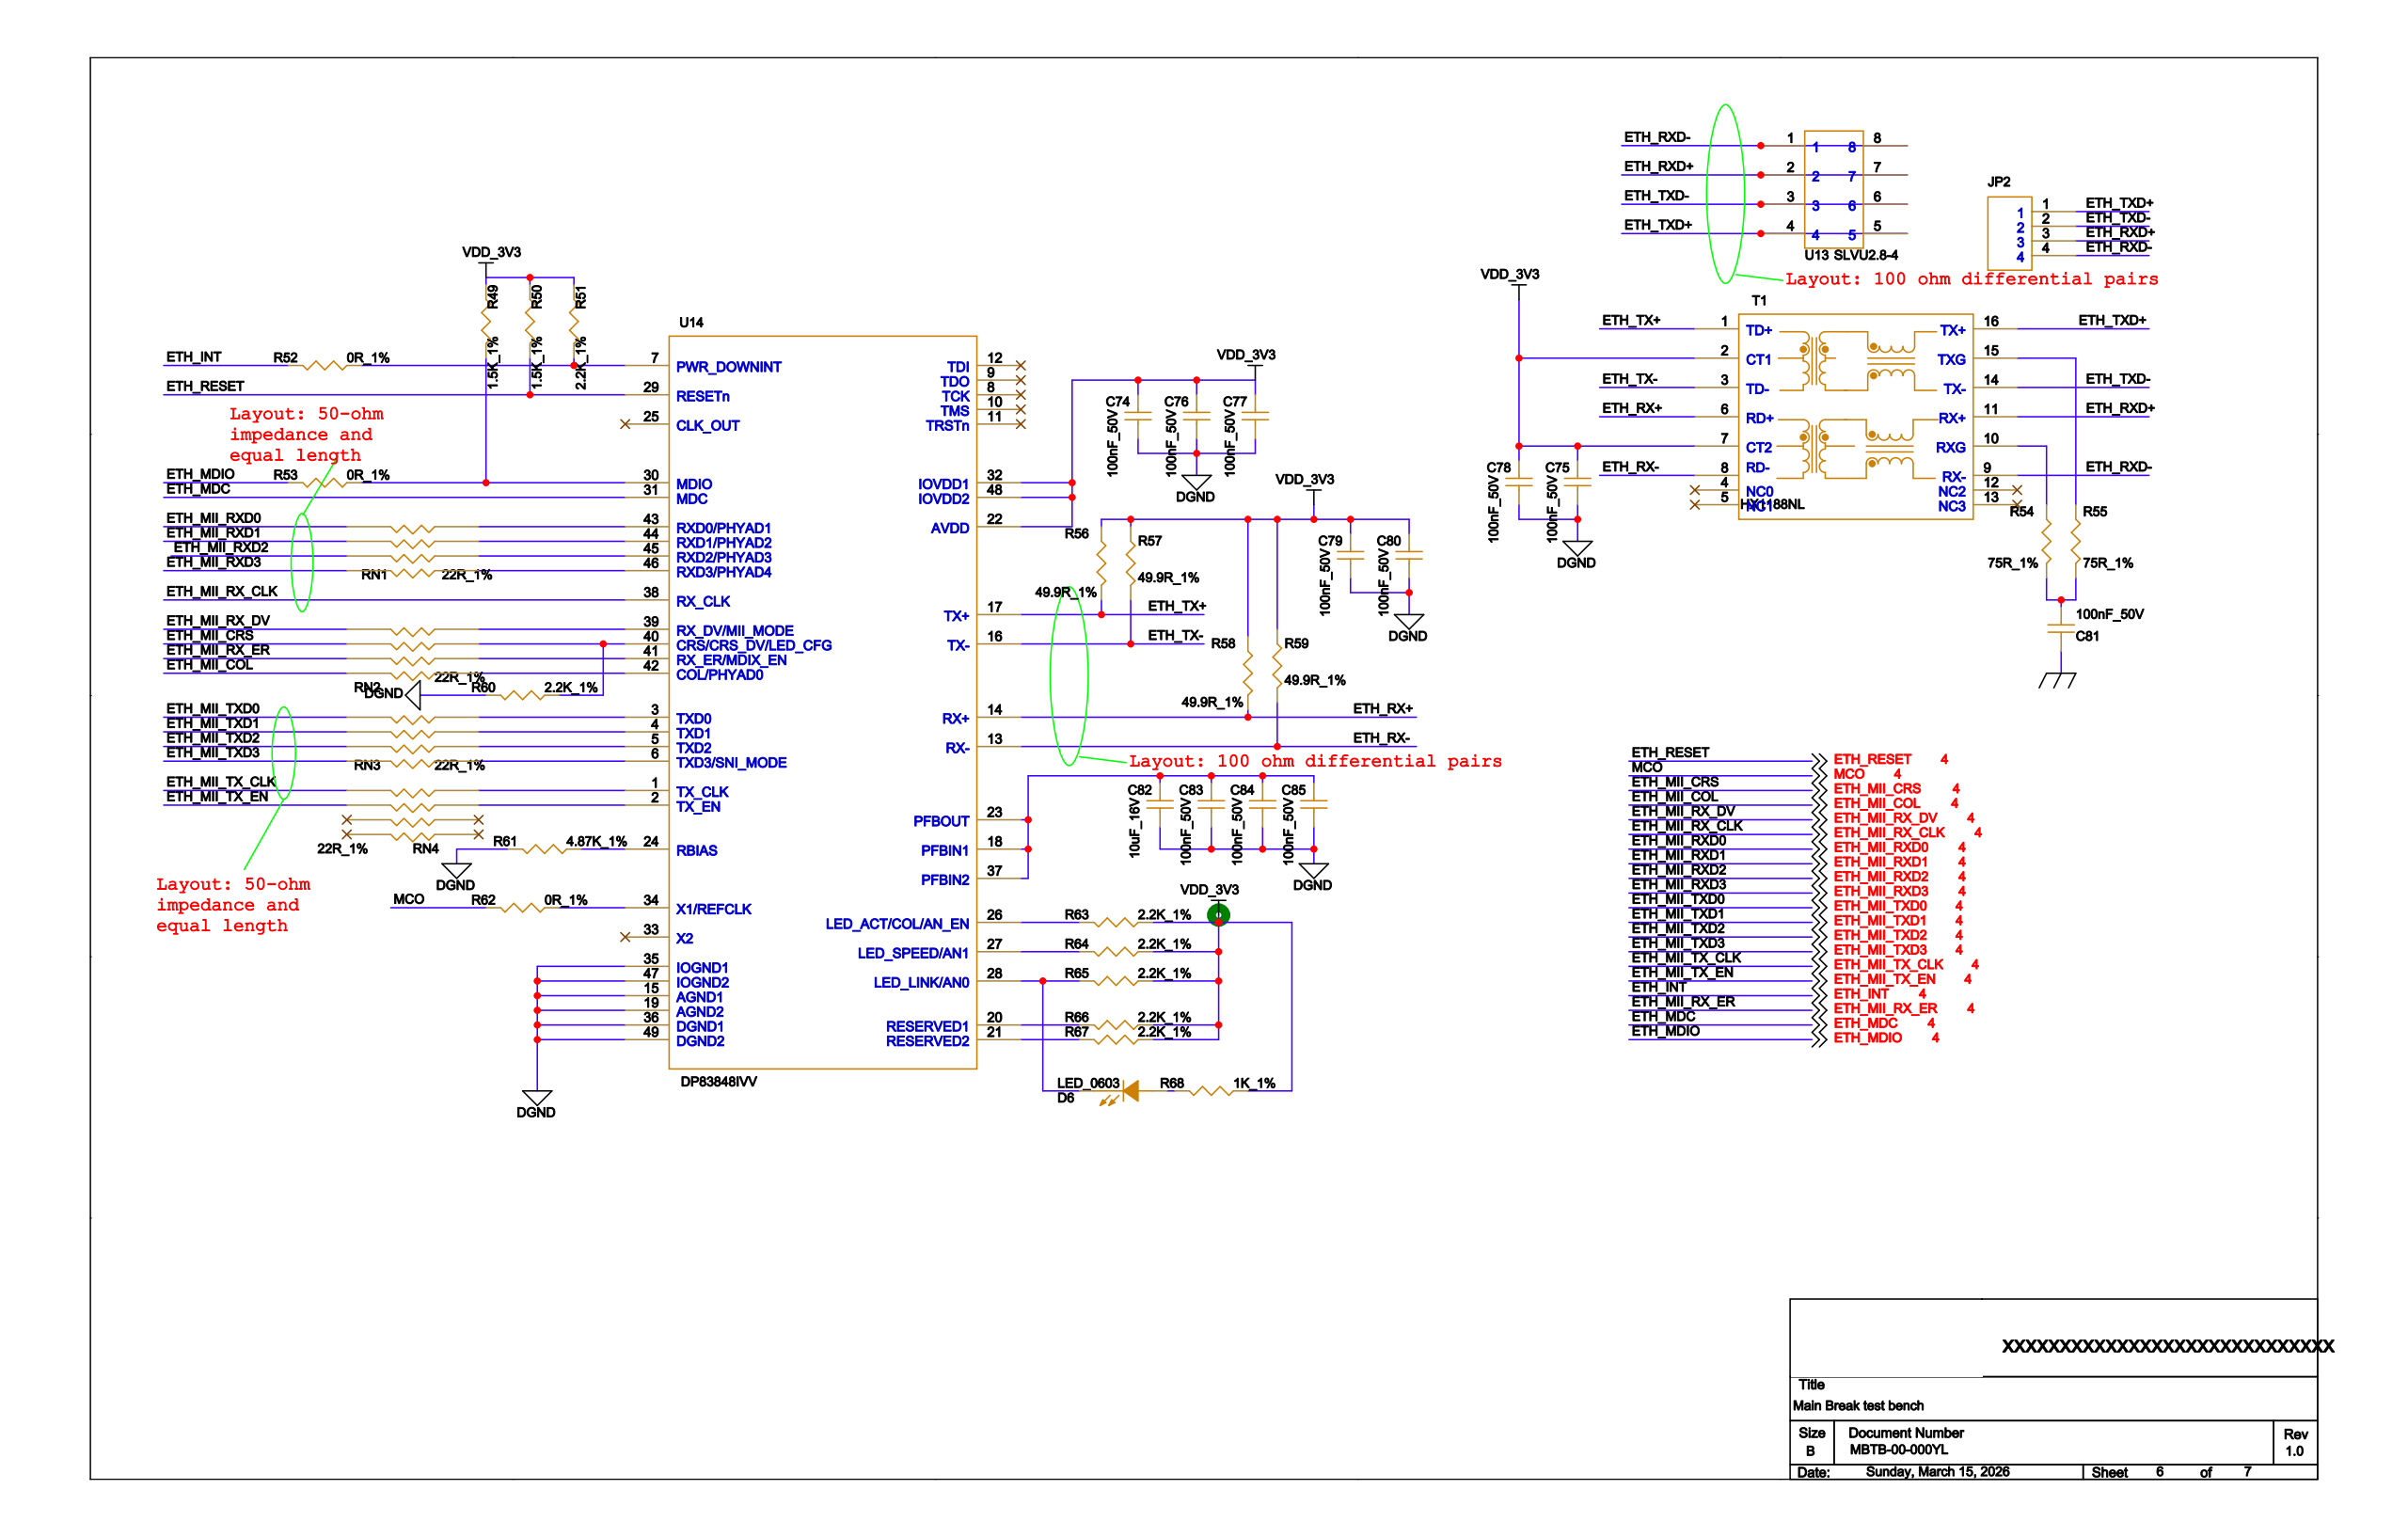Circuit board | Cadence Allegro | 260 parts | 211 nets | one sheet of the schematic
Parts on this sheet (reference | value | footprint):
C81 | 0603-C
JP2 | 21033814412
R49 | 0603-R
R50 | 0603-R
R51 | 0603-R
R52 | 0603-R
R53 | 0603-R
R54 | 0603-R
R55 | 0603-R
R56 | 0603-R
R57 | 0603-R
R58 | 0603-R
R59 | 0603-R
R60 | 0603-R
R61 | 0603-R
R62 | 0603-R
R63 | 0603-R
R64 | 0603-R
R65 | 0603-R
R66 | 0603-R
R67 | 0603-R
R68 | 0603-R
RN1 | RN0603
RN2 | RN0603
RN3 | RN0603
RN4 | RN0603
T1 | TFM16-1_27-7_11-5_97
U13 | SOIC8-1_27-5_1X4_0-H1_75
U14 | QFP_48
Nets of these parts (net: part-pin ...):
VDD_3V3: R49-2 R50-2 R51-2 R56-2 R57-2 R58-2 R59-2 R63-2 R64-2 R65-2 R66-2 R67-2 R68-2 T1-2 T1-7 U14-22 U14-32 U14-48
DGND: R60-1 R61-1 U14-15 U14-19 U14-35 U14-36 U14-47 U14-49
N16790298: C81-1 R54-1 R55-1
GND_EARTH: C81-2
N16789542: R65-1 U14-28
N16790256: R68-1
ETH_TXD+: JP2-1 T1-16 U13-4 U13-5
ETH_TXD-: JP2-2 T1-14 U13-3 U13-6
ETH_RXD+: JP2-3 T1-11 U13-2 U13-7
ETH_RXD-: JP2-4 T1-9 U13-1 U13-8
N16789212: R49-1 R53-2 U14-30
ETH_RESET: R50-1 U14-29
N16789274: R51-1 R52-2 U14-7
N16789244: R60-2 RN2-3 U14-40
N16789530: R63-1 U14-26
N16789540: R64-1 U14-27
N16789544: R66-1 U14-20
N16789546: R67-1 U14-21
ETH_INT: R52-1
ETH_MDIO: R53-1
MCO: R62-1
N16789199: R62-2 U14-34
N16790200: R54-2 T1-10
N16790204: R55-2 T1-15
ETH_TX+: R56-1 T1-1 U14-17
ETH_TX-: R57-1 T1-3 U14-16
ETH_RX+: R58-1 T1-6 U14-14
ETH_RX-: R59-1 T1-8 U14-13
N16789422: R61-2 U14-24
N16790117: RN1-1 U14-46
N16790119: RN1-2 U14-45
N16790121: RN1-3 U14-44
N16790123: RN1-4
ETH_MII_RXD0: RN1-5
ETH_MII_RXD1: RN1-6
ETH_MII_RXD2: RN1-7
ETH_MII_RXD3: RN1-8
N16790125: RN2-1 U14-42
N16790152: RN2-2 U14-41
N16790154: RN2-4 U14-39
ETH_MII_RX_DV: RN2-5
ETH_MII_CRS: RN2-6
ETH_MII_RX_ER: RN2-7
ETH_MII_COL: RN2-8
N16790111: RN3-1 U14-6
N16790113: RN3-2 U14-5
N16790115: RN3-3 U14-4
N16790109: RN3-4 U14-3
ETH_MII_TXD0: RN3-5
ETH_MII_TXD1: RN3-6
ETH_MII_TXD2: RN3-7
ETH_MII_TXD3: RN3-8
N16790246: RN4-3 U14-2
N16790244: RN4-4 U14-1
ETH_MII_TX_CLK: RN4-5
ETH_MII_TX_EN: RN4-6
ETH_MDC: U14-31
ETH_MII_RX_CLK: U14-38